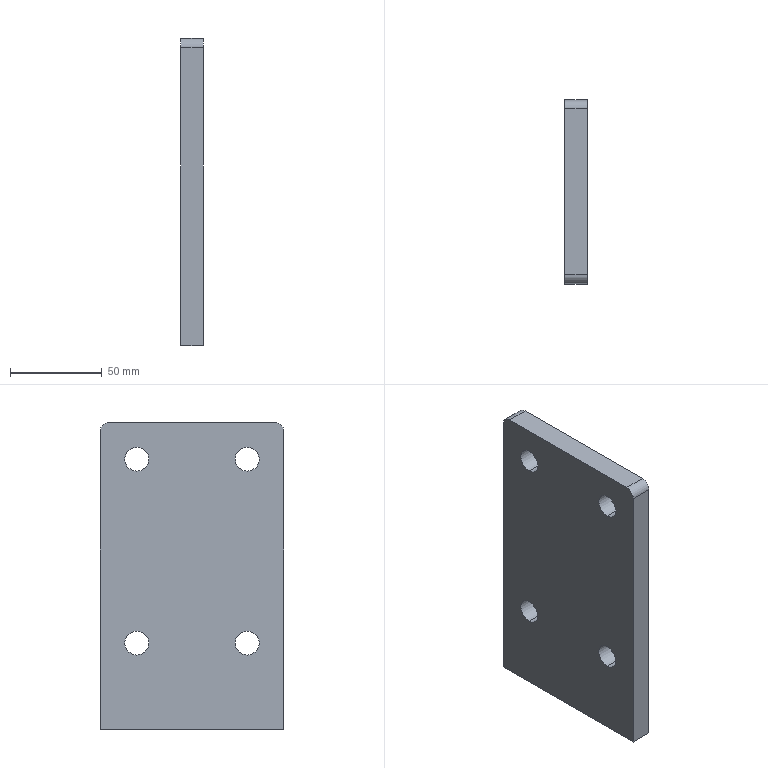Part | STEP file | 1 solid | 16 faces | box 12 x 100 x 167 mm | volume 193900 mm3 | cylinder 10 | plane 6 | commonest cylinder face diameters 13 x8 10 x2
STEP:
#1=CARTESIAN_POINT('',(0.,0.,0.));
#2=DIRECTION('',(0.,0.,1.));
#3=DIRECTION('',(1.,0.,0.));
#4=AXIS2_PLACEMENT_3D('',#1,#2,#3);
#5=CARTESIAN_POINT('',(-227.,-1110.,53.5));
#6=VERTEX_POINT('',#5);
#7=CARTESIAN_POINT('',(-227.,-1110.,40.5));
#8=VERTEX_POINT('',#7);
#9=CARTESIAN_POINT('',(-227.,-1110.,47.));
#10=DIRECTION('',(1.,0.,0.));
#11=DIRECTION('',(0.,0.,1.));
#12=AXIS2_PLACEMENT_3D('',#9,#10,#11);
#13=CIRCLE('',#12,6.5);
#14=CARTESIAN_POINT('',(-227.,-1030.,167.));
#15=DIRECTION('',(1.,0.,0.));
#16=DIRECTION('',(0.,1.,0.));
#17=AXIS2_PLACEMENT_3D('',#14,#15,#16);
#18=PLANE('',#17);
#19=CARTESIAN_POINT('',(-80.,-120.));
#20=DIRECTION('',(0.,1.));
#21=AXIS2_PLACEMENT_2D('',#19,#20);
#22=CIRCLE('',#21,6.5);
#23=(GEOMETRIC_REPRESENTATION_CONTEXT(2)PARAMETRIC_REPRESENTATION_CONTEXT()REPRESENTATION_CONTEXT('',''));
#24=DEFINITIONAL_REPRESENTATION('',(#22),#23);
#25=PCURVE('',#18,#24);
#26=CARTESIAN_POINT('',(-214.999,-1110.,47.));
#27=DIRECTION('',(-1.,0.,0.));
#28=DIRECTION('',(0.,0.,1.));
#29=AXIS2_PLACEMENT_3D('',#26,#27,#28);
#30=CYLINDRICAL_SURFACE('',#29,6.5);
#31=CARTESIAN_POINT('',(6.283,12.001));
#32=DIRECTION('',(-1.,0.));
#33=VECTOR('',#32,1.);
#34=LINE('',#31,#33);
#35=(GEOMETRIC_REPRESENTATION_CONTEXT(2)PARAMETRIC_REPRESENTATION_CONTEXT()REPRESENTATION_CONTEXT('',''));
#36=DEFINITIONAL_REPRESENTATION('',(#34),#35);
#37=PCURVE('',#30,#36);
#38=SURFACE_CURVE('',#13,(#25,#37),.PCURVE_S1.);
#39=EDGE_CURVE('',#6,#8,#38,.T.);
#40=ORIENTED_EDGE('',*,*,#39,.T.);
#41=CARTESIAN_POINT('',(-227.,-1110.,47.));
#42=DIRECTION('',(1.,0.,0.));
#43=DIRECTION('',(0.,0.,1.));
#44=AXIS2_PLACEMENT_3D('',#41,#42,#43);
#45=CIRCLE('',#44,6.5);
#46=CARTESIAN_POINT('',(-80.,-120.));
#47=DIRECTION('',(0.,1.));
#48=AXIS2_PLACEMENT_2D('',#46,#47);
#49=CIRCLE('',#48,6.5);
#50=(GEOMETRIC_REPRESENTATION_CONTEXT(2)PARAMETRIC_REPRESENTATION_CONTEXT()REPRESENTATION_CONTEXT('',''));
#51=DEFINITIONAL_REPRESENTATION('',(#49),#50);
#52=PCURVE('',#18,#51);
#53=CARTESIAN_POINT('',(-214.999,-1110.,47.));
#54=DIRECTION('',(-1.,0.,0.));
#55=DIRECTION('',(0.,0.,1.));
#56=AXIS2_PLACEMENT_3D('',#53,#54,#55);
#57=CYLINDRICAL_SURFACE('',#56,6.5);
#58=CARTESIAN_POINT('',(6.283,12.001));
#59=DIRECTION('',(-1.,0.));
#60=VECTOR('',#59,1.);
#61=LINE('',#58,#60);
#62=(GEOMETRIC_REPRESENTATION_CONTEXT(2)PARAMETRIC_REPRESENTATION_CONTEXT()REPRESENTATION_CONTEXT('',''));
#63=DEFINITIONAL_REPRESENTATION('',(#61),#62);
#64=PCURVE('',#57,#63);
#65=SURFACE_CURVE('',#45,(#52,#64),.PCURVE_S1.);
#66=EDGE_CURVE('',#8,#6,#65,.T.);
#67=ORIENTED_EDGE('',*,*,#66,.T.);
#68=EDGE_LOOP('',(#40,#67));
#69=FACE_BOUND('',#68,.T.);
#70=CARTESIAN_POINT('',(-227.,-1110.,153.5));
#71=VERTEX_POINT('',#70);
#72=CARTESIAN_POINT('',(-227.,-1110.,140.5));
#73=VERTEX_POINT('',#72);
#74=CARTESIAN_POINT('',(-227.,-1110.,147.));
#75=DIRECTION('',(1.,0.,0.));
#76=DIRECTION('',(0.,0.,1.));
#77=AXIS2_PLACEMENT_3D('',#74,#75,#76);
#78=CIRCLE('',#77,6.5);
#79=CARTESIAN_POINT('',(-80.,-20.));
#80=DIRECTION('',(0.,1.));
#81=AXIS2_PLACEMENT_2D('',#79,#80);
#82=CIRCLE('',#81,6.5);
#83=(GEOMETRIC_REPRESENTATION_CONTEXT(2)PARAMETRIC_REPRESENTATION_CONTEXT()REPRESENTATION_CONTEXT('',''));
#84=DEFINITIONAL_REPRESENTATION('',(#82),#83);
#85=PCURVE('',#18,#84);
#86=CARTESIAN_POINT('',(-214.999,-1110.,147.));
#87=DIRECTION('',(-1.,0.,0.));
#88=DIRECTION('',(0.,0.,1.));
#89=AXIS2_PLACEMENT_3D('',#86,#87,#88);
#90=CYLINDRICAL_SURFACE('',#89,6.5);
#91=CARTESIAN_POINT('',(6.283,12.001));
#92=DIRECTION('',(-1.,0.));
#93=VECTOR('',#92,1.);
#94=LINE('',#91,#93);
#95=(GEOMETRIC_REPRESENTATION_CONTEXT(2)PARAMETRIC_REPRESENTATION_CONTEXT()REPRESENTATION_CONTEXT('',''));
#96=DEFINITIONAL_REPRESENTATION('',(#94),#95);
#97=PCURVE('',#90,#96);
#98=SURFACE_CURVE('',#78,(#85,#97),.PCURVE_S1.);
#99=EDGE_CURVE('',#71,#73,#98,.T.);
#100=ORIENTED_EDGE('',*,*,#99,.T.);
#101=CARTESIAN_POINT('',(-227.,-1110.,147.));
#102=DIRECTION('',(1.,0.,0.));
#103=DIRECTION('',(0.,0.,1.));
#104=AXIS2_PLACEMENT_3D('',#101,#102,#103);
#105=CIRCLE('',#104,6.5);
#106=CARTESIAN_POINT('',(-80.,-20.));
#107=DIRECTION('',(0.,1.));
#108=AXIS2_PLACEMENT_2D('',#106,#107);
#109=CIRCLE('',#108,6.5);
#110=(GEOMETRIC_REPRESENTATION_CONTEXT(2)PARAMETRIC_REPRESENTATION_CONTEXT()REPRESENTATION_CONTEXT('',''));
#111=DEFINITIONAL_REPRESENTATION('',(#109),#110);
#112=PCURVE('',#18,#111);
#113=CARTESIAN_POINT('',(-214.999,-1110.,147.));
#114=DIRECTION('',(-1.,0.,0.));
#115=DIRECTION('',(0.,0.,1.));
#116=AXIS2_PLACEMENT_3D('',#113,#114,#115);
#117=CYLINDRICAL_SURFACE('',#116,6.5);
#118=CARTESIAN_POINT('',(6.283,12.001));
#119=DIRECTION('',(-1.,0.));
#120=VECTOR('',#119,1.);
#121=LINE('',#118,#120);
#122=(GEOMETRIC_REPRESENTATION_CONTEXT(2)PARAMETRIC_REPRESENTATION_CONTEXT()REPRESENTATION_CONTEXT('',''));
#123=DEFINITIONAL_REPRESENTATION('',(#121),#122);
#124=PCURVE('',#117,#123);
#125=SURFACE_CURVE('',#105,(#112,#124),.PCURVE_S1.);
#126=EDGE_CURVE('',#73,#71,#125,.T.);
#127=ORIENTED_EDGE('',*,*,#126,.T.);
#128=EDGE_LOOP('',(#100,#127));
#129=FACE_BOUND('',#128,.T.);
#130=CARTESIAN_POINT('',(-227.,-1050.,153.5));
#131=VERTEX_POINT('',#130);
#132=CARTESIAN_POINT('',(-227.,-1050.,140.5));
#133=VERTEX_POINT('',#132);
#134=CARTESIAN_POINT('',(-227.,-1050.,147.));
#135=DIRECTION('',(1.,0.,0.));
#136=DIRECTION('',(0.,0.,1.));
#137=AXIS2_PLACEMENT_3D('',#134,#135,#136);
#138=CIRCLE('',#137,6.5);
#139=CARTESIAN_POINT('',(-20.,-20.));
#140=DIRECTION('',(0.,1.));
#141=AXIS2_PLACEMENT_2D('',#139,#140);
#142=CIRCLE('',#141,6.5);
#143=(GEOMETRIC_REPRESENTATION_CONTEXT(2)PARAMETRIC_REPRESENTATION_CONTEXT()REPRESENTATION_CONTEXT('',''));
#144=DEFINITIONAL_REPRESENTATION('',(#142),#143);
#145=PCURVE('',#18,#144);
#146=CARTESIAN_POINT('',(-214.999,-1050.,147.));
#147=DIRECTION('',(-1.,0.,0.));
#148=DIRECTION('',(0.,0.,1.));
#149=AXIS2_PLACEMENT_3D('',#146,#147,#148);
#150=CYLINDRICAL_SURFACE('',#149,6.5);
#151=CARTESIAN_POINT('',(6.283,12.001));
#152=DIRECTION('',(-1.,0.));
#153=VECTOR('',#152,1.);
#154=LINE('',#151,#153);
#155=(GEOMETRIC_REPRESENTATION_CONTEXT(2)PARAMETRIC_REPRESENTATION_CONTEXT()REPRESENTATION_CONTEXT('',''));
#156=DEFINITIONAL_REPRESENTATION('',(#154),#155);
#157=PCURVE('',#150,#156);
#158=SURFACE_CURVE('',#138,(#145,#157),.PCURVE_S1.);
#159=EDGE_CURVE('',#131,#133,#158,.T.);
#160=ORIENTED_EDGE('',*,*,#159,.T.);
#161=CARTESIAN_POINT('',(-227.,-1050.,147.));
#162=DIRECTION('',(1.,0.,0.));
#163=DIRECTION('',(0.,0.,1.));
#164=AXIS2_PLACEMENT_3D('',#161,#162,#163);
#165=CIRCLE('',#164,6.5);
#166=CARTESIAN_POINT('',(-20.,-20.));
#167=DIRECTION('',(0.,1.));
#168=AXIS2_PLACEMENT_2D('',#166,#167);
#169=CIRCLE('',#168,6.5);
#170=(GEOMETRIC_REPRESENTATION_CONTEXT(2)PARAMETRIC_REPRESENTATION_CONTEXT()REPRESENTATION_CONTEXT('',''));
#171=DEFINITIONAL_REPRESENTATION('',(#169),#170);
#172=PCURVE('',#18,#171);
#173=CARTESIAN_POINT('',(-214.999,-1050.,147.));
#174=DIRECTION('',(-1.,0.,0.));
#175=DIRECTION('',(0.,0.,1.));
#176=AXIS2_PLACEMENT_3D('',#173,#174,#175);
#177=CYLINDRICAL_SURFACE('',#176,6.5);
#178=CARTESIAN_POINT('',(6.283,12.001));
#179=DIRECTION('',(-1.,0.));
#180=VECTOR('',#179,1.);
#181=LINE('',#178,#180);
#182=(GEOMETRIC_REPRESENTATION_CONTEXT(2)PARAMETRIC_REPRESENTATION_CONTEXT()REPRESENTATION_CONTEXT('',''));
#183=DEFINITIONAL_REPRESENTATION('',(#181),#182);
#184=PCURVE('',#177,#183);
#185=SURFACE_CURVE('',#165,(#172,#184),.PCURVE_S1.);
#186=EDGE_CURVE('',#133,#131,#185,.T.);
#187=ORIENTED_EDGE('',*,*,#186,.T.);
#188=EDGE_LOOP('',(#160,#187));
#189=FACE_BOUND('',#188,.T.);
#190=CARTESIAN_POINT('',(-227.,-1050.,53.5));
#191=VERTEX_POINT('',#190);
#192=CARTESIAN_POINT('',(-227.,-1050.,40.5));
#193=VERTEX_POINT('',#192);
#194=CARTESIAN_POINT('',(-227.,-1050.,47.));
#195=DIRECTION('',(1.,0.,0.));
#196=DIRECTION('',(0.,0.,1.));
#197=AXIS2_PLACEMENT_3D('',#194,#195,#196);
#198=CIRCLE('',#197,6.5);
#199=CARTESIAN_POINT('',(-20.,-120.));
#200=DIRECTION('',(0.,1.));
#201=AXIS2_PLACEMENT_2D('',#199,#200);
#202=CIRCLE('',#201,6.5);
#203=(GEOMETRIC_REPRESENTATION_CONTEXT(2)PARAMETRIC_REPRESENTATION_CONTEXT()REPRESENTATION_CONTEXT('',''));
#204=DEFINITIONAL_REPRESENTATION('',(#202),#203);
#205=PCURVE('',#18,#204);
#206=CARTESIAN_POINT('',(-214.999,-1050.,47.));
#207=DIRECTION('',(-1.,0.,0.));
#208=DIRECTION('',(0.,0.,1.));
#209=AXIS2_PLACEMENT_3D('',#206,#207,#208);
#210=CYLINDRICAL_SURFACE('',#209,6.5);
#211=CARTESIAN_POINT('',(6.283,12.001));
#212=DIRECTION('',(-1.,0.));
#213=VECTOR('',#212,1.);
#214=LINE('',#211,#213);
#215=(GEOMETRIC_REPRESENTATION_CONTEXT(2)PARAMETRIC_REPRESENTATION_CONTEXT()REPRESENTATION_CONTEXT('',''));
#216=DEFINITIONAL_REPRESENTATION('',(#214),#215);
#217=PCURVE('',#210,#216);
#218=SURFACE_CURVE('',#198,(#205,#217),.PCURVE_S1.);
#219=EDGE_CURVE('',#191,#193,#218,.T.);
#220=ORIENTED_EDGE('',*,*,#219,.T.);
#221=CARTESIAN_POINT('',(-227.,-1050.,47.));
#222=DIRECTION('',(1.,0.,0.));
#223=DIRECTION('',(0.,0.,1.));
#224=AXIS2_PLACEMENT_3D('',#221,#222,#223);
#225=CIRCLE('',#224,6.5);
#226=CARTESIAN_POINT('',(-20.,-120.));
#227=DIRECTION('',(0.,1.));
#228=AXIS2_PLACEMENT_2D('',#226,#227);
#229=CIRCLE('',#228,6.5);
#230=(GEOMETRIC_REPRESENTATION_CONTEXT(2)PARAMETRIC_REPRESENTATION_CONTEXT()REPRESENTATION_CONTEXT('',''));
#231=DEFINITIONAL_REPRESENTATION('',(#229),#230);
#232=PCURVE('',#18,#231);
#233=CARTESIAN_POINT('',(-214.999,-1050.,47.));
#234=DIRECTION('',(-1.,0.,0.));
#235=DIRECTION('',(0.,0.,1.));
#236=AXIS2_PLACEMENT_3D('',#233,#234,#235);
#237=CYLINDRICAL_SURFACE('',#236,6.5);
#238=CARTESIAN_POINT('',(6.283,12.001));
#239=DIRECTION('',(-1.,0.));
#240=VECTOR('',#239,1.);
#241=LINE('',#238,#240);
#242=(GEOMETRIC_REPRESENTATION_CONTEXT(2)PARAMETRIC_REPRESENTATION_CONTEXT()REPRESENTATION_CONTEXT('',''));
#243=DEFINITIONAL_REPRESENTATION('',(#241),#242);
#244=PCURVE('',#237,#243);
#245=SURFACE_CURVE('',#225,(#232,#244),.PCURVE_S1.);
#246=EDGE_CURVE('',#193,#191,#245,.T.);
#247=ORIENTED_EDGE('',*,*,#246,.T.);
#248=EDGE_LOOP('',(#220,#247));
#249=FACE_BOUND('',#248,.T.);
#250=CARTESIAN_POINT('',(-227.,-1125.,167.));
#251=VERTEX_POINT('',#250);
#252=CARTESIAN_POINT('',(-227.,-1130.,162.));
#253=VERTEX_POINT('',#252);
#254=CARTESIAN_POINT('',(-227.,-1125.,162.));
#255=DIRECTION('',(1.,0.,0.));
#256=DIRECTION('',(0.,0.,1.));
#257=AXIS2_PLACEMENT_3D('',#254,#255,#256);
#258=CIRCLE('',#257,5.);
#259=CARTESIAN_POINT('',(-95.,-5.));
#260=DIRECTION('',(0.,1.));
#261=AXIS2_PLACEMENT_2D('',#259,#260);
#262=CIRCLE('',#261,5.);
#263=(GEOMETRIC_REPRESENTATION_CONTEXT(2)PARAMETRIC_REPRESENTATION_CONTEXT()REPRESENTATION_CONTEXT('',''));
#264=DEFINITIONAL_REPRESENTATION('',(#262),#263);
#265=PCURVE('',#18,#264);
#266=CARTESIAN_POINT('',(0.,-1125.,162.));
#267=DIRECTION('',(-1.,0.,0.));
#268=DIRECTION('',(0.,0.,1.));
#269=AXIS2_PLACEMENT_3D('',#266,#267,#268);
#270=CYLINDRICAL_SURFACE('',#269,5.);
#271=CARTESIAN_POINT('',(6.283,227.));
#272=DIRECTION('',(-1.,0.));
#273=VECTOR('',#272,1.);
#274=LINE('',#271,#273);
#275=(GEOMETRIC_REPRESENTATION_CONTEXT(2)PARAMETRIC_REPRESENTATION_CONTEXT()REPRESENTATION_CONTEXT('',''));
#276=DEFINITIONAL_REPRESENTATION('',(#274),#275);
#277=PCURVE('',#270,#276);
#278=SURFACE_CURVE('',#258,(#265,#277),.PCURVE_S1.);
#279=EDGE_CURVE('',#251,#253,#278,.T.);
#280=ORIENTED_EDGE('',*,*,#279,.F.);
#281=CARTESIAN_POINT('',(-227.,-1035.,167.));
#282=VERTEX_POINT('',#281);
#283=CARTESIAN_POINT('',(-227.,0.,167.));
#284=DIRECTION('',(0.,-1.,0.));
#285=VECTOR('',#284,1.);
#286=LINE('',#283,#285);
#287=CARTESIAN_POINT('',(1030.,0.));
#288=DIRECTION('',(-1.,0.));
#289=VECTOR('',#288,1.);
#290=LINE('',#287,#289);
#291=(GEOMETRIC_REPRESENTATION_CONTEXT(2)PARAMETRIC_REPRESENTATION_CONTEXT()REPRESENTATION_CONTEXT('',''));
#292=DEFINITIONAL_REPRESENTATION('',(#290),#291);
#293=PCURVE('',#18,#292);
#294=CARTESIAN_POINT('',(0.,0.,167.));
#295=DIRECTION('',(0.,0.,1.));
#296=DIRECTION('',(1.,0.,0.));
#297=AXIS2_PLACEMENT_3D('',#294,#295,#296);
#298=PLANE('',#297);
#299=CARTESIAN_POINT('',(-227.,0.));
#300=DIRECTION('',(0.,-1.));
#301=VECTOR('',#300,1.);
#302=LINE('',#299,#301);
#303=(GEOMETRIC_REPRESENTATION_CONTEXT(2)PARAMETRIC_REPRESENTATION_CONTEXT()REPRESENTATION_CONTEXT('',''));
#304=DEFINITIONAL_REPRESENTATION('',(#302),#303);
#305=PCURVE('',#298,#304);
#306=SURFACE_CURVE('',#286,(#293,#305),.PCURVE_S1.);
#307=EDGE_CURVE('',#282,#251,#306,.T.);
#308=ORIENTED_EDGE('',*,*,#307,.F.);
#309=CARTESIAN_POINT('',(-227.,-1030.,162.));
#310=VERTEX_POINT('',#309);
#311=CARTESIAN_POINT('',(-227.,-1035.,162.));
#312=DIRECTION('',(1.,0.,0.));
#313=DIRECTION('',(0.,0.,-1.));
#314=AXIS2_PLACEMENT_3D('',#311,#312,#313);
#315=CIRCLE('',#314,5.);
#316=CARTESIAN_POINT('',(-5.,-5.));
#317=DIRECTION('',(0.,-1.));
#318=AXIS2_PLACEMENT_2D('',#316,#317);
#319=CIRCLE('',#318,5.);
#320=(GEOMETRIC_REPRESENTATION_CONTEXT(2)PARAMETRIC_REPRESENTATION_CONTEXT()REPRESENTATION_CONTEXT('',''));
#321=DEFINITIONAL_REPRESENTATION('',(#319),#320);
#322=PCURVE('',#18,#321);
#323=CARTESIAN_POINT('',(0.,-1035.,162.));
#324=DIRECTION('',(1.,0.,0.));
#325=DIRECTION('',(0.,0.,-1.));
#326=AXIS2_PLACEMENT_3D('',#323,#324,#325);
#327=CYLINDRICAL_SURFACE('',#326,5.);
#328=CARTESIAN_POINT('',(0.,-227.));
#329=DIRECTION('',(1.,0.));
#330=VECTOR('',#329,1.);
#331=LINE('',#328,#330);
#332=(GEOMETRIC_REPRESENTATION_CONTEXT(2)PARAMETRIC_REPRESENTATION_CONTEXT()REPRESENTATION_CONTEXT('',''));
#333=DEFINITIONAL_REPRESENTATION('',(#331),#332);
#334=PCURVE('',#327,#333);
#335=SURFACE_CURVE('',#315,(#322,#334),.PCURVE_S1.);
#336=EDGE_CURVE('',#310,#282,#335,.T.);
#337=ORIENTED_EDGE('',*,*,#336,.F.);
#338=CARTESIAN_POINT('',(-227.,-1030.,0.));
#339=VERTEX_POINT('',#338);
#340=CARTESIAN_POINT('',(-227.,-1030.,167.));
#341=DIRECTION('',(0.,0.,-1.));
#342=VECTOR('',#341,1.);
#343=LINE('',#340,#342);
#344=CARTESIAN_POINT('',(0.,0.));
#345=DIRECTION('',(0.,-1.));
#346=VECTOR('',#345,1.);
#347=LINE('',#344,#346);
#348=(GEOMETRIC_REPRESENTATION_CONTEXT(2)PARAMETRIC_REPRESENTATION_CONTEXT()REPRESENTATION_CONTEXT('',''));
#349=DEFINITIONAL_REPRESENTATION('',(#347),#348);
#350=PCURVE('',#18,#349);
#351=CARTESIAN_POINT('',(-227.,-1030.,167.));
#352=DIRECTION('',(0.,-1.,0.));
#353=DIRECTION('',(0.,0.,-1.));
#354=AXIS2_PLACEMENT_3D('',#351,#352,#353);
#355=PLANE('',#354);
#356=CARTESIAN_POINT('',(0.,0.));
#357=DIRECTION('',(1.,0.));
#358=VECTOR('',#357,1.);
#359=LINE('',#356,#358);
#360=(GEOMETRIC_REPRESENTATION_CONTEXT(2)PARAMETRIC_REPRESENTATION_CONTEXT()REPRESENTATION_CONTEXT('',''));
#361=DEFINITIONAL_REPRESENTATION('',(#359),#360);
#362=PCURVE('',#355,#361);
#363=SURFACE_CURVE('',#343,(#350,#362),.PCURVE_S1.);
#364=EDGE_CURVE('',#310,#339,#363,.T.);
#365=ORIENTED_EDGE('',*,*,#364,.T.);
#366=CARTESIAN_POINT('',(-227.,-1130.,0.));
#367=VERTEX_POINT('',#366);
#368=CARTESIAN_POINT('',(-227.,0.,0.));
#369=DIRECTION('',(0.,-1.,0.));
#370=VECTOR('',#369,1.);
#371=LINE('',#368,#370);
#372=CARTESIAN_POINT('',(1030.,-167.));
#373=DIRECTION('',(-1.,0.));
#374=VECTOR('',#373,1.);
#375=LINE('',#372,#374);
#376=(GEOMETRIC_REPRESENTATION_CONTEXT(2)PARAMETRIC_REPRESENTATION_CONTEXT()REPRESENTATION_CONTEXT('',''));
#377=DEFINITIONAL_REPRESENTATION('',(#375),#376);
#378=PCURVE('',#18,#377);
#379=CARTESIAN_POINT('',(0.,0.,0.));
#380=DIRECTION('',(0.,0.,1.));
#381=DIRECTION('',(1.,0.,0.));
#382=AXIS2_PLACEMENT_3D('',#379,#380,#381);
#383=PLANE('',#382);
#384=CARTESIAN_POINT('',(-227.,0.));
#385=DIRECTION('',(0.,-1.));
#386=VECTOR('',#385,1.);
#387=LINE('',#384,#386);
#388=(GEOMETRIC_REPRESENTATION_CONTEXT(2)PARAMETRIC_REPRESENTATION_CONTEXT()REPRESENTATION_CONTEXT('',''));
#389=DEFINITIONAL_REPRESENTATION('',(#387),#388);
#390=PCURVE('',#383,#389);
#391=SURFACE_CURVE('',#371,(#378,#390),.PCURVE_S1.);
#392=EDGE_CURVE('',#339,#367,#391,.T.);
#393=ORIENTED_EDGE('',*,*,#392,.T.);
#394=CARTESIAN_POINT('',(-227.,-1130.,167.));
#395=DIRECTION('',(0.,0.,1.));
#396=VECTOR('',#395,1.);
#397=LINE('',#394,#396);
#398=CARTESIAN_POINT('',(-100.,0.));
#399=DIRECTION('',(0.,1.));
#400=VECTOR('',#399,1.);
#401=LINE('',#398,#400);
#402=(GEOMETRIC_REPRESENTATION_CONTEXT(2)PARAMETRIC_REPRESENTATION_CONTEXT()REPRESENTATION_CONTEXT('',''));
#403=DEFINITIONAL_REPRESENTATION('',(#401),#402);
#404=PCURVE('',#18,#403);
#405=CARTESIAN_POINT('',(-227.,-1130.,167.));
#406=DIRECTION('',(0.,1.,0.));
#407=DIRECTION('',(1.,0.,0.));
#408=AXIS2_PLACEMENT_3D('',#405,#406,#407);
#409=PLANE('',#408);
#410=CARTESIAN_POINT('',(0.,0.));
#411=DIRECTION('',(0.,-1.));
#412=VECTOR('',#411,1.);
#413=LINE('',#410,#412);
#414=(GEOMETRIC_REPRESENTATION_CONTEXT(2)PARAMETRIC_REPRESENTATION_CONTEXT()REPRESENTATION_CONTEXT('',''));
#415=DEFINITIONAL_REPRESENTATION('',(#413),#414);
#416=PCURVE('',#409,#415);
#417=SURFACE_CURVE('',#397,(#404,#416),.PCURVE_S1.);
#418=EDGE_CURVE('',#367,#253,#417,.T.);
#419=ORIENTED_EDGE('',*,*,#418,.T.);
#420=EDGE_LOOP('',(#280,#308,#337,#365,#393,#419));
#421=FACE_BOUND('',#420,.T.);
#422=ADVANCED_FACE('',(#69,#129,#189,#249,#421),#18,.F.);
#423=ORIENTED_EDGE('',*,*,#66,.T.);
#424=CARTESIAN_POINT('',(-215.,-1110.,53.5));
#425=VERTEX_POINT('',#424);
#426=CARTESIAN_POINT('',(-214.999,-1110.,53.5));
#427=DIRECTION('',(-1.,0.,0.));
#428=VECTOR('',#427,1.);
#429=LINE('',#426,#428);
#430=CARTESIAN_POINT('',(0.,0.));
#431=DIRECTION('',(0.,1.));
#432=VECTOR('',#431,1.);
#433=LINE('',#430,#432);
#434=(GEOMETRIC_REPRESENTATION_CONTEXT(2)PARAMETRIC_REPRESENTATION_CONTEXT()REPRESENTATION_CONTEXT('',''));
#435=DEFINITIONAL_REPRESENTATION('',(#433),#434);
#436=PCURVE('',#57,#435);
#437=CARTESIAN_POINT('',(6.283,0.));
#438=DIRECTION('',(0.,1.));
#439=VECTOR('',#438,1.);
#440=LINE('',#437,#439);
#441=(GEOMETRIC_REPRESENTATION_CONTEXT(2)PARAMETRIC_REPRESENTATION_CONTEXT()REPRESENTATION_CONTEXT('',''));
#442=DEFINITIONAL_REPRESENTATION('',(#440),#441);
#443=PCURVE('',#30,#442);
#444=SURFACE_CURVE('',#429,(#436,#443),.PCURVE_S1.);
#445=EDGE_CURVE('',#425,#6,#444,.T.);
#446=ORIENTED_EDGE('',*,*,#445,.F.);
#447=CARTESIAN_POINT('',(-215.,-1110.,40.5));
#448=VERTEX_POINT('',#447);
#449=CARTESIAN_POINT('',(-215.,-1110.,47.));
#450=DIRECTION('',(1.,0.,0.));
#451=DIRECTION('',(0.,0.,1.));
#452=AXIS2_PLACEMENT_3D('',#449,#450,#451);
#453=CIRCLE('',#452,6.5);
#454=CARTESIAN_POINT('',(6.283,0.001));
#455=DIRECTION('',(-1.,0.));
#456=VECTOR('',#455,1.);
#457=LINE('',#454,#456);
#458=(GEOMETRIC_REPRESENTATION_CONTEXT(2)PARAMETRIC_REPRESENTATION_CONTEXT()REPRESENTATION_CONTEXT('',''));
#459=DEFINITIONAL_REPRESENTATION('',(#457),#458);
#460=PCURVE('',#57,#459);
#461=CARTESIAN_POINT('',(-215.,-1030.,167.));
#462=DIRECTION('',(-1.,0.,0.));
#463=DIRECTION('',(0.,0.,1.));
#464=AXIS2_PLACEMENT_3D('',#461,#462,#463);
#465=PLANE('',#464);
#466=CARTESIAN_POINT('',(-113.5,-80.));
#467=CARTESIAN_POINT('',(-113.5,-91.258));
#468=CARTESIAN_POINT('',(-123.25,-85.629));
#469=CARTESIAN_POINT('',(-133.,-80.));
#470=CARTESIAN_POINT('',(-123.25,-74.371));
#471=CARTESIAN_POINT('',(-113.5,-68.742));
#472=CARTESIAN_POINT('',(-113.5,-80.));
#473=(BOUNDED_CURVE()B_SPLINE_CURVE(2,(#466,#467,#468,#469,#470,#471,#472),.UNSPECIFIED.,.T.,.F.)B_SPLINE_CURVE_WITH_KNOTS((1,2,2,2,2,1),(-2.094,0.,2.094,4.189,6.283,8.378),.UNSPECIFIED.)CURVE()GEOMETRIC_REPRESENTATION_ITEM()RATIONAL_B_SPLINE_CURVE((1.,0.5,1.,0.5,1.,0.5,1.))REPRESENTATION_ITEM(''));
#474=(GEOMETRIC_REPRESENTATION_CONTEXT(2)PARAMETRIC_REPRESENTATION_CONTEXT()REPRESENTATION_CONTEXT('',''));
#475=DEFINITIONAL_REPRESENTATION('',(#473),#474);
#476=PCURVE('',#465,#475);
#477=SURFACE_CURVE('',#453,(#460,#476),.PCURVE_S1.);
#478=EDGE_CURVE('',#448,#425,#477,.T.);
#479=ORIENTED_EDGE('',*,*,#478,.F.);
#480=CARTESIAN_POINT('',(-214.999,-1110.,40.5));
#481=DIRECTION('',(-1.,0.,0.));
#482=VECTOR('',#481,1.);
#483=LINE('',#480,#482);
#484=CARTESIAN_POINT('',(3.142,0.));
#485=DIRECTION('',(0.,1.));
#486=VECTOR('',#485,1.);
#487=LINE('',#484,#486);
#488=(GEOMETRIC_REPRESENTATION_CONTEXT(2)PARAMETRIC_REPRESENTATION_CONTEXT()REPRESENTATION_CONTEXT('',''));
#489=DEFINITIONAL_REPRESENTATION('',(#487),#488);
#490=PCURVE('',#57,#489);
#491=CARTESIAN_POINT('',(3.142,0.));
#492=DIRECTION('',(0.,1.));
#493=VECTOR('',#492,1.);
#494=LINE('',#491,#493);
#495=(GEOMETRIC_REPRESENTATION_CONTEXT(2)PARAMETRIC_REPRESENTATION_CONTEXT()REPRESENTATION_CONTEXT('',''));
#496=DEFINITIONAL_REPRESENTATION('',(#494),#495);
#497=PCURVE('',#30,#496);
#498=SURFACE_CURVE('',#483,(#490,#497),.PCURVE_S1.);
#499=EDGE_CURVE('',#448,#8,#498,.T.);
#500=ORIENTED_EDGE('',*,*,#499,.T.);
#501=EDGE_LOOP('',(#423,#446,#479,#500));
#502=FACE_BOUND('',#501,.F.);
#503=ADVANCED_FACE('',(#502),#57,.F.);
#504=ORIENTED_EDGE('',*,*,#126,.T.);
#505=CARTESIAN_POINT('',(-215.,-1110.,153.5));
#506=VERTEX_POINT('',#505);
#507=CARTESIAN_POINT('',(-214.999,-1110.,153.5));
#508=DIRECTION('',(-1.,0.,0.));
#509=VECTOR('',#508,1.);
#510=LINE('',#507,#509);
#511=CARTESIAN_POINT('',(0.,0.));
#512=DIRECTION('',(0.,1.));
#513=VECTOR('',#512,1.);
#514=LINE('',#511,#513);
#515=(GEOMETRIC_REPRESENTATION_CONTEXT(2)PARAMETRIC_REPRESENTATION_CONTEXT()REPRESENTATION_CONTEXT('',''));
#516=DEFINITIONAL_REPRESENTATION('',(#514),#515);
#517=PCURVE('',#117,#516);
#518=CARTESIAN_POINT('',(6.283,0.));
#519=DIRECTION('',(0.,1.));
#520=VECTOR('',#519,1.);
#521=LINE('',#518,#520);
#522=(GEOMETRIC_REPRESENTATION_CONTEXT(2)PARAMETRIC_REPRESENTATION_CONTEXT()REPRESENTATION_CONTEXT('',''));
#523=DEFINITIONAL_REPRESENTATION('',(#521),#522);
#524=PCURVE('',#90,#523);
#525=SURFACE_CURVE('',#510,(#517,#524),.PCURVE_S1.);
#526=EDGE_CURVE('',#506,#71,#525,.T.);
#527=ORIENTED_EDGE('',*,*,#526,.F.);
#528=CARTESIAN_POINT('',(-215.,-1110.,140.5));
#529=VERTEX_POINT('',#528);
#530=CARTESIAN_POINT('',(-215.,-1110.,147.));
#531=DIRECTION('',(1.,0.,0.));
#532=DIRECTION('',(0.,0.,1.));
#533=AXIS2_PLACEMENT_3D('',#530,#531,#532);
#534=CIRCLE('',#533,6.5);
#535=CARTESIAN_POINT('',(6.283,0.001));
#536=DIRECTION('',(-1.,0.));
#537=VECTOR('',#536,1.);
#538=LINE('',#535,#537);
#539=(GEOMETRIC_REPRESENTATION_CONTEXT(2)PARAMETRIC_REPRESENTATION_CONTEXT()REPRESENTATION_CONTEXT('',''));
#540=DEFINITIONAL_REPRESENTATION('',(#538),#539);
#541=PCURVE('',#117,#540);
#542=CARTESIAN_POINT('',(-13.5,-80.));
#543=CARTESIAN_POINT('',(-13.5,-91.258));
#544=CARTESIAN_POINT('',(-23.25,-85.629));
#545=CARTESIAN_POINT('',(-33.,-80.));
#546=CARTESIAN_POINT('',(-23.25,-74.371));
#547=CARTESIAN_POINT('',(-13.5,-68.742));
#548=CARTESIAN_POINT('',(-13.5,-80.));
#549=(BOUNDED_CURVE()B_SPLINE_CURVE(2,(#542,#543,#544,#545,#546,#547,#548),.UNSPECIFIED.,.T.,.F.)B_SPLINE_CURVE_WITH_KNOTS((1,2,2,2,2,1),(-2.094,0.,2.094,4.189,6.283,8.378),.UNSPECIFIED.)CURVE()GEOMETRIC_REPRESENTATION_ITEM()RATIONAL_B_SPLINE_CURVE((1.,0.5,1.,0.5,1.,0.5,1.))REPRESENTATION_ITEM(''));
#550=(GEOMETRIC_REPRESENTATION_CONTEXT(2)PARAMETRIC_REPRESENTATION_CONTEXT()REPRESENTATION_CONTEXT('',''));
#551=DEFINITIONAL_REPRESENTATION('',(#549),#550);
#552=PCURVE('',#465,#551);
#553=SURFACE_CURVE('',#534,(#541,#552),.PCURVE_S1.);
#554=EDGE_CURVE('',#529,#506,#553,.T.);
#555=ORIENTED_EDGE('',*,*,#554,.F.);
#556=CARTESIAN_POINT('',(-214.999,-1110.,140.5));
#557=DIRECTION('',(-1.,0.,0.));
#558=VECTOR('',#557,1.);
#559=LINE('',#556,#558);
#560=CARTESIAN_POINT('',(3.142,0.));
#561=DIRECTION('',(0.,1.));
#562=VECTOR('',#561,1.);
#563=LINE('',#560,#562);
#564=(GEOMETRIC_REPRESENTATION_CONTEXT(2)PARAMETRIC_REPRESENTATION_CONTEXT()REPRESENTATION_CONTEXT('',''));
#565=DEFINITIONAL_REPRESENTATION('',(#563),#564);
#566=PCURVE('',#117,#565);
#567=CARTESIAN_POINT('',(3.142,0.));
#568=DIRECTION('',(0.,1.));
#569=VECTOR('',#568,1.);
#570=LINE('',#567,#569);
#571=(GEOMETRIC_REPRESENTATION_CONTEXT(2)PARAMETRIC_REPRESENTATION_CONTEXT()REPRESENTATION_CONTEXT('',''));
#572=DEFINITIONAL_REPRESENTATION('',(#570),#571);
#573=PCURVE('',#90,#572);
#574=SURFACE_CURVE('',#559,(#566,#573),.PCURVE_S1.);
#575=EDGE_CURVE('',#529,#73,#574,.T.);
#576=ORIENTED_EDGE('',*,*,#575,.T.);
#577=EDGE_LOOP('',(#504,#527,#555,#576));
#578=FACE_BOUND('',#577,.F.);
#579=ADVANCED_FACE('',(#578),#117,.F.);
#580=ORIENTED_EDGE('',*,*,#186,.T.);
#581=CARTESIAN_POINT('',(-215.,-1050.,153.5));
#582=VERTEX_POINT('',#581);
#583=CARTESIAN_POINT('',(-214.999,-1050.,153.5));
#584=DIRECTION('',(-1.,0.,0.));
#585=VECTOR('',#584,1.);
#586=LINE('',#583,#585);
#587=CARTESIAN_POINT('',(0.,0.));
#588=DIRECTION('',(0.,1.));
#589=VECTOR('',#588,1.);
#590=LINE('',#587,#589);
#591=(GEOMETRIC_REPRESENTATION_CONTEXT(2)PARAMETRIC_REPRESENTATION_CONTEXT()REPRESENTATION_CONTEXT('',''));
#592=DEFINITIONAL_REPRESENTATION('',(#590),#591);
#593=PCURVE('',#177,#592);
#594=CARTESIAN_POINT('',(6.283,0.));
#595=DIRECTION('',(0.,1.));
#596=VECTOR('',#595,1.);
#597=LINE('',#594,#596);
#598=(GEOMETRIC_REPRESENTATION_CONTEXT(2)PARAMETRIC_REPRESENTATION_CONTEXT()REPRESENTATION_CONTEXT('',''));
#599=DEFINITIONAL_REPRESENTATION('',(#597),#598);
#600=PCURVE('',#150,#599);
#601=SURFACE_CURVE('',#586,(#593,#600),.PCURVE_S1.);
#602=EDGE_CURVE('',#582,#131,#601,.T.);
#603=ORIENTED_EDGE('',*,*,#602,.F.);
#604=CARTESIAN_POINT('',(-215.,-1050.,140.5));
#605=VERTEX_POINT('',#604);
#606=CARTESIAN_POINT('',(-215.,-1050.,147.));
#607=DIRECTION('',(1.,0.,0.));
#608=DIRECTION('',(0.,0.,1.));
#609=AXIS2_PLACEMENT_3D('',#606,#607,#608);
#610=CIRCLE('',#609,6.5);
#611=CARTESIAN_POINT('',(6.283,0.001));
#612=DIRECTION('',(-1.,0.));
#613=VECTOR('',#612,1.);
#614=LINE('',#611,#613);
#615=(GEOMETRIC_REPRESENTATION_CONTEXT(2)PARAMETRIC_REPRESENTATION_CONTEXT()REPRESENTATION_CONTEXT('',''));
#616=DEFINITIONAL_REPRESENTATION('',(#614),#615);
#617=PCURVE('',#177,#616);
#618=CARTESIAN_POINT('',(-13.5,-20.));
#619=CARTESIAN_POINT('',(-13.5,-31.258));
#620=CARTESIAN_POINT('',(-23.25,-25.629));
#621=CARTESIAN_POINT('',(-33.,-20.));
#622=CARTESIAN_POINT('',(-23.25,-14.371));
#623=CARTESIAN_POINT('',(-13.5,-8.742));
#624=CARTESIAN_POINT('',(-13.5,-20.));
#625=(BOUNDED_CURVE()B_SPLINE_CURVE(2,(#618,#619,#620,#621,#622,#623,#624),.UNSPECIFIED.,.T.,.F.)B_SPLINE_CURVE_WITH_KNOTS((1,2,2,2,2,1),(-2.094,0.,2.094,4.189,6.283,8.378),.UNSPECIFIED.)CURVE()GEOMETRIC_REPRESENTATION_ITEM()RATIONAL_B_SPLINE_CURVE((1.,0.5,1.,0.5,1.,0.5,1.))REPRESENTATION_ITEM(''));
#626=(GEOMETRIC_REPRESENTATION_CONTEXT(2)PARAMETRIC_REPRESENTATION_CONTEXT()REPRESENTATION_CONTEXT('',''));
#627=DEFINITIONAL_REPRESENTATION('',(#625),#626);
#628=PCURVE('',#465,#627);
#629=SURFACE_CURVE('',#610,(#617,#628),.PCURVE_S1.);
#630=EDGE_CURVE('',#605,#582,#629,.T.);
#631=ORIENTED_EDGE('',*,*,#630,.F.);
#632=CARTESIAN_POINT('',(-214.999,-1050.,140.5));
#633=DIRECTION('',(-1.,0.,0.));
#634=VECTOR('',#633,1.);
#635=LINE('',#632,#634);
#636=CARTESIAN_POINT('',(3.142,0.));
#637=DIRECTION('',(0.,1.));
#638=VECTOR('',#637,1.);
#639=LINE('',#636,#638);
#640=(GEOMETRIC_REPRESENTATION_CONTEXT(2)PARAMETRIC_REPRESENTATION_CONTEXT()REPRESENTATION_CONTEXT('',''));
#641=DEFINITIONAL_REPRESENTATION('',(#639),#640);
#642=PCURVE('',#177,#641);
#643=CARTESIAN_POINT('',(3.142,0.));
#644=DIRECTION('',(0.,1.));
#645=VECTOR('',#644,1.);
#646=LINE('',#643,#645);
#647=(GEOMETRIC_REPRESENTATION_CONTEXT(2)PARAMETRIC_REPRESENTATION_CONTEXT()REPRESENTATION_CONTEXT('',''));
#648=DEFINITIONAL_REPRESENTATION('',(#646),#647);
#649=PCURVE('',#150,#648);
#650=SURFACE_CURVE('',#635,(#642,#649),.PCURVE_S1.);
#651=EDGE_CURVE('',#605,#133,#650,.T.);
#652=ORIENTED_EDGE('',*,*,#651,.T.);
#653=EDGE_LOOP('',(#580,#603,#631,#652));
#654=FACE_BOUND('',#653,.F.);
#655=ADVANCED_FACE('',(#654),#177,.F.);
#656=ORIENTED_EDGE('',*,*,#246,.T.);
#657=CARTESIAN_POINT('',(-215.,-1050.,53.5));
#658=VERTEX_POINT('',#657);
#659=CARTESIAN_POINT('',(-214.999,-1050.,53.5));
#660=DIRECTION('',(-1.,0.,0.));
#661=VECTOR('',#660,1.);
#662=LINE('',#659,#661);
#663=CARTESIAN_POINT('',(0.,0.));
#664=DIRECTION('',(0.,1.));
#665=VECTOR('',#664,1.);
#666=LINE('',#663,#665);
#667=(GEOMETRIC_REPRESENTATION_CONTEXT(2)PARAMETRIC_REPRESENTATION_CONTEXT()REPRESENTATION_CONTEXT('',''));
#668=DEFINITIONAL_REPRESENTATION('',(#666),#667);
#669=PCURVE('',#237,#668);
#670=CARTESIAN_POINT('',(6.283,0.));
#671=DIRECTION('',(0.,1.));
#672=VECTOR('',#671,1.);
#673=LINE('',#670,#672);
#674=(GEOMETRIC_REPRESENTATION_CONTEXT(2)PARAMETRIC_REPRESENTATION_CONTEXT()REPRESENTATION_CONTEXT('',''));
#675=DEFINITIONAL_REPRESENTATION('',(#673),#674);
#676=PCURVE('',#210,#675);
#677=SURFACE_CURVE('',#662,(#669,#676),.PCURVE_S1.);
#678=EDGE_CURVE('',#658,#191,#677,.T.);
#679=ORIENTED_EDGE('',*,*,#678,.F.);
#680=CARTESIAN_POINT('',(-215.,-1050.,40.5));
#681=VERTEX_POINT('',#680);
#682=CARTESIAN_POINT('',(-215.,-1050.,47.));
#683=DIRECTION('',(1.,0.,0.));
#684=DIRECTION('',(0.,0.,1.));
#685=AXIS2_PLACEMENT_3D('',#682,#683,#684);
#686=CIRCLE('',#685,6.5);
#687=CARTESIAN_POINT('',(6.283,0.001));
#688=DIRECTION('',(-1.,0.));
#689=VECTOR('',#688,1.);
#690=LINE('',#687,#689);
#691=(GEOMETRIC_REPRESENTATION_CONTEXT(2)PARAMETRIC_REPRESENTATION_CONTEXT()REPRESENTATION_CONTEXT('',''));
#692=DEFINITIONAL_REPRESENTATION('',(#690),#691);
#693=PCURVE('',#237,#692);
#694=CARTESIAN_POINT('',(-113.5,-20.));
#695=CARTESIAN_POINT('',(-113.5,-31.258));
#696=CARTESIAN_POINT('',(-123.25,-25.629));
#697=CARTESIAN_POINT('',(-133.,-20.));
#698=CARTESIAN_POINT('',(-123.25,-14.371));
#699=CARTESIAN_POINT('',(-113.5,-8.742));
#700=CARTESIAN_POINT('',(-113.5,-20.));
#701=(BOUNDED_CURVE()B_SPLINE_CURVE(2,(#694,#695,#696,#697,#698,#699,#700),.UNSPECIFIED.,.T.,.F.)B_SPLINE_CURVE_WITH_KNOTS((1,2,2,2,2,1),(-2.094,0.,2.094,4.189,6.283,8.378),.UNSPECIFIED.)CURVE()GEOMETRIC_REPRESENTATION_ITEM()RATIONAL_B_SPLINE_CURVE((1.,0.5,1.,0.5,1.,0.5,1.))REPRESENTATION_ITEM(''));
#702=(GEOMETRIC_REPRESENTATION_CONTEXT(2)PARAMETRIC_REPRESENTATION_CONTEXT()REPRESENTATION_CONTEXT('',''));
#703=DEFINITIONAL_REPRESENTATION('',(#701),#702);
#704=PCURVE('',#465,#703);
#705=SURFACE_CURVE('',#686,(#693,#704),.PCURVE_S1.);
#706=EDGE_CURVE('',#681,#658,#705,.T.);
#707=ORIENTED_EDGE('',*,*,#706,.F.);
#708=CARTESIAN_POINT('',(-214.999,-1050.,40.5));
#709=DIRECTION('',(-1.,0.,0.));
#710=VECTOR('',#709,1.);
#711=LINE('',#708,#710);
#712=CARTESIAN_POINT('',(3.142,0.));
#713=DIRECTION('',(0.,1.));
#714=VECTOR('',#713,1.);
#715=LINE('',#712,#714);
#716=(GEOMETRIC_REPRESENTATION_CONTEXT(2)PARAMETRIC_REPRESENTATION_CONTEXT()REPRESENTATION_CONTEXT('',''));
#717=DEFINITIONAL_REPRESENTATION('',(#715),#716);
#718=PCURVE('',#237,#717);
#719=CARTESIAN_POINT('',(3.142,0.));
#720=DIRECTION('',(0.,1.));
#721=VECTOR('',#720,1.);
#722=LINE('',#719,#721);
#723=(GEOMETRIC_REPRESENTATION_CONTEXT(2)PARAMETRIC_REPRESENTATION_CONTEXT()REPRESENTATION_CONTEXT('',''));
#724=DEFINITIONAL_REPRESENTATION('',(#722),#723);
#725=PCURVE('',#210,#724);
#726=SURFACE_CURVE('',#711,(#718,#725),.PCURVE_S1.);
#727=EDGE_CURVE('',#681,#193,#726,.T.);
#728=ORIENTED_EDGE('',*,*,#727,.T.);
#729=EDGE_LOOP('',(#656,#679,#707,#728));
#730=FACE_BOUND('',#729,.F.);
#731=ADVANCED_FACE('',(#730),#237,.F.);
#732=ORIENTED_EDGE('',*,*,#336,.T.);
#733=CARTESIAN_POINT('',(-215.,-1035.,167.));
#734=VERTEX_POINT('',#733);
#735=CARTESIAN_POINT('',(0.,-1035.,167.));
#736=DIRECTION('',(-1.,0.,0.));
#737=VECTOR('',#736,1.);
#738=LINE('',#735,#737);
#739=CARTESIAN_POINT('',(3.142,0.));
#740=DIRECTION('',(0.,-1.));
#741=VECTOR('',#740,1.);
#742=LINE('',#739,#741);
#743=(GEOMETRIC_REPRESENTATION_CONTEXT(2)PARAMETRIC_REPRESENTATION_CONTEXT()REPRESENTATION_CONTEXT('',''));
#744=DEFINITIONAL_REPRESENTATION('',(#742),#743);
#745=PCURVE('',#327,#744);
#746=CARTESIAN_POINT('',(0.,-1035.));
#747=DIRECTION('',(-1.,0.));
#748=VECTOR('',#747,1.);
#749=LINE('',#746,#748);
#750=(GEOMETRIC_REPRESENTATION_CONTEXT(2)PARAMETRIC_REPRESENTATION_CONTEXT()REPRESENTATION_CONTEXT('',''));
#751=DEFINITIONAL_REPRESENTATION('',(#749),#750);
#752=PCURVE('',#298,#751);
#753=SURFACE_CURVE('',#738,(#745,#752),.PCURVE_S1.);
#754=EDGE_CURVE('',#734,#282,#753,.T.);
#755=ORIENTED_EDGE('',*,*,#754,.F.);
#756=CARTESIAN_POINT('',(-215.,-1030.,162.));
#757=VERTEX_POINT('',#756);
#758=CARTESIAN_POINT('',(-215.,-1035.,162.));
#759=DIRECTION('',(-1.,0.,0.));
#760=DIRECTION('',(0.,0.,-1.));
#761=AXIS2_PLACEMENT_3D('',#758,#759,#760);
#762=CIRCLE('',#761,5.);
#763=CARTESIAN_POINT('',(6.283,-215.));
#764=DIRECTION('',(-1.,0.));
#765=VECTOR('',#764,1.);
#766=LINE('',#763,#765);
#767=(GEOMETRIC_REPRESENTATION_CONTEXT(2)PARAMETRIC_REPRESENTATION_CONTEXT()REPRESENTATION_CONTEXT('',''));
#768=DEFINITIONAL_REPRESENTATION('',(#766),#767);
#769=PCURVE('',#327,#768);
#770=CARTESIAN_POINT('',(-5.,-5.));
#771=DIRECTION('',(-1.,0.));
#772=AXIS2_PLACEMENT_2D('',#770,#771);
#773=CIRCLE('',#772,5.);
#774=(GEOMETRIC_REPRESENTATION_CONTEXT(2)PARAMETRIC_REPRESENTATION_CONTEXT()REPRESENTATION_CONTEXT('',''));
#775=DEFINITIONAL_REPRESENTATION('',(#773),#774);
#776=PCURVE('',#465,#775);
#777=SURFACE_CURVE('',#762,(#769,#776),.PCURVE_S1.);
#778=EDGE_CURVE('',#734,#757,#777,.T.);
#779=ORIENTED_EDGE('',*,*,#778,.T.);
#780=CARTESIAN_POINT('',(-227.,-1030.,162.));
#781=DIRECTION('',(-1.,0.,0.));
#782=VECTOR('',#781,1.);
#783=LINE('',#780,#782);
#784=CARTESIAN_POINT('',(1.571,-227.));
#785=DIRECTION('',(0.,-1.));
#786=VECTOR('',#785,1.);
#787=LINE('',#784,#786);
#788=(GEOMETRIC_REPRESENTATION_CONTEXT(2)PARAMETRIC_REPRESENTATION_CONTEXT()REPRESENTATION_CONTEXT('',''));
#789=DEFINITIONAL_REPRESENTATION('',(#787),#788);
#790=PCURVE('',#327,#789);
#791=CARTESIAN_POINT('',(5.,0.));
#792=DIRECTION('',(0.,-1.));
#793=VECTOR('',#792,1.);
#794=LINE('',#791,#793);
#795=(GEOMETRIC_REPRESENTATION_CONTEXT(2)PARAMETRIC_REPRESENTATION_CONTEXT()REPRESENTATION_CONTEXT('',''));
#796=DEFINITIONAL_REPRESENTATION('',(#794),#795);
#797=PCURVE('',#355,#796);
#798=SURFACE_CURVE('',#783,(#790,#797),.PCURVE_S1.);
#799=EDGE_CURVE('',#757,#310,#798,.T.);
#800=ORIENTED_EDGE('',*,*,#799,.T.);
#801=EDGE_LOOP('',(#732,#755,#779,#800));
#802=FACE_BOUND('',#801,.T.);
#803=ADVANCED_FACE('',(#802),#327,.T.);
#804=ORIENTED_EDGE('',*,*,#799,.F.);
#805=CARTESIAN_POINT('',(-215.,-1030.,0.));
#806=VERTEX_POINT('',#805);
#807=CARTESIAN_POINT('',(-215.,-1030.,167.));
#808=DIRECTION('',(0.,0.,-1.));
#809=VECTOR('',#808,1.);
#810=LINE('',#807,#809);
#811=CARTESIAN_POINT('',(0.,12.));
#812=DIRECTION('',(1.,0.));
#813=VECTOR('',#812,1.);
#814=LINE('',#811,#813);
#815=(GEOMETRIC_REPRESENTATION_CONTEXT(2)PARAMETRIC_REPRESENTATION_CONTEXT()REPRESENTATION_CONTEXT('',''));
#816=DEFINITIONAL_REPRESENTATION('',(#814),#815);
#817=PCURVE('',#355,#816);
#818=CARTESIAN_POINT('',(0.,0.));
#819=DIRECTION('',(-1.,0.));
#820=VECTOR('',#819,1.);
#821=LINE('',#818,#820);
#822=(GEOMETRIC_REPRESENTATION_CONTEXT(2)PARAMETRIC_REPRESENTATION_CONTEXT()REPRESENTATION_CONTEXT('',''));
#823=DEFINITIONAL_REPRESENTATION('',(#821),#822);
#824=PCURVE('',#465,#823);
#825=SURFACE_CURVE('',#810,(#817,#824),.PCURVE_S1.);
#826=EDGE_CURVE('',#757,#806,#825,.T.);
#827=ORIENTED_EDGE('',*,*,#826,.T.);
#828=CARTESIAN_POINT('',(0.,-1030.,0.));
#829=DIRECTION('',(-1.,0.,0.));
#830=VECTOR('',#829,1.);
#831=LINE('',#828,#830);
#832=CARTESIAN_POINT('',(167.,227.));
#833=DIRECTION('',(0.,-1.));
#834=VECTOR('',#833,1.);
#835=LINE('',#832,#834);
#836=(GEOMETRIC_REPRESENTATION_CONTEXT(2)PARAMETRIC_REPRESENTATION_CONTEXT()REPRESENTATION_CONTEXT('',''));
#837=DEFINITIONAL_REPRESENTATION('',(#835),#836);
#838=PCURVE('',#355,#837);
#839=CARTESIAN_POINT('',(0.,-1030.));
#840=DIRECTION('',(-1.,0.));
#841=VECTOR('',#840,1.);
#842=LINE('',#839,#841);
#843=(GEOMETRIC_REPRESENTATION_CONTEXT(2)PARAMETRIC_REPRESENTATION_CONTEXT()REPRESENTATION_CONTEXT('',''));
#844=DEFINITIONAL_REPRESENTATION('',(#842),#843);
#845=PCURVE('',#383,#844);
#846=SURFACE_CURVE('',#831,(#838,#845),.PCURVE_S1.);
#847=EDGE_CURVE('',#806,#339,#846,.T.);
#848=ORIENTED_EDGE('',*,*,#847,.T.);
#849=ORIENTED_EDGE('',*,*,#364,.F.);
#850=EDGE_LOOP('',(#804,#827,#848,#849));
#851=FACE_BOUND('',#850,.T.);
#852=ADVANCED_FACE('',(#851),#355,.F.);
#853=ORIENTED_EDGE('',*,*,#847,.F.);
#854=CARTESIAN_POINT('',(-215.,-1130.,0.));
#855=VERTEX_POINT('',#854);
#856=CARTESIAN_POINT('',(-215.,-1030.,0.));
#857=DIRECTION('',(0.,-1.,0.));
#858=VECTOR('',#857,1.);
#859=LINE('',#856,#858);
#860=CARTESIAN_POINT('',(-215.,-1030.));
#861=DIRECTION('',(0.,-1.));
#862=VECTOR('',#861,1.);
#863=LINE('',#860,#862);
#864=(GEOMETRIC_REPRESENTATION_CONTEXT(2)PARAMETRIC_REPRESENTATION_CONTEXT()REPRESENTATION_CONTEXT('',''));
#865=DEFINITIONAL_REPRESENTATION('',(#863),#864);
#866=PCURVE('',#383,#865);
#867=CARTESIAN_POINT('',(-167.,0.));
#868=DIRECTION('',(0.,-1.));
#869=VECTOR('',#868,1.);
#870=LINE('',#867,#869);
#871=(GEOMETRIC_REPRESENTATION_CONTEXT(2)PARAMETRIC_REPRESENTATION_CONTEXT()REPRESENTATION_CONTEXT('',''));
#872=DEFINITIONAL_REPRESENTATION('',(#870),#871);
#873=PCURVE('',#465,#872);
#874=SURFACE_CURVE('',#859,(#866,#873),.PCURVE_S1.);
#875=EDGE_CURVE('',#806,#855,#874,.T.);
#876=ORIENTED_EDGE('',*,*,#875,.T.);
#877=CARTESIAN_POINT('',(-227.,-1130.,0.));
#878=DIRECTION('',(-1.,0.,0.));
#879=VECTOR('',#878,1.);
#880=LINE('',#877,#879);
#881=CARTESIAN_POINT('',(-227.,-1130.));
#882=DIRECTION('',(-1.,0.));
#883=VECTOR('',#882,1.);
#884=LINE('',#881,#883);
#885=(GEOMETRIC_REPRESENTATION_CONTEXT(2)PARAMETRIC_REPRESENTATION_CONTEXT()REPRESENTATION_CONTEXT('',''));
#886=DEFINITIONAL_REPRESENTATION('',(#884),#885);
#887=PCURVE('',#383,#886);
#888=CARTESIAN_POINT('',(0.,167.));
#889=DIRECTION('',(-1.,0.));
#890=VECTOR('',#889,1.);
#891=LINE('',#888,#890);
#892=(GEOMETRIC_REPRESENTATION_CONTEXT(2)PARAMETRIC_REPRESENTATION_CONTEXT()REPRESENTATION_CONTEXT('',''));
#893=DEFINITIONAL_REPRESENTATION('',(#891),#892);
#894=PCURVE('',#409,#893);
#895=SURFACE_CURVE('',#880,(#887,#894),.PCURVE_S1.);
#896=EDGE_CURVE('',#855,#367,#895,.T.);
#897=ORIENTED_EDGE('',*,*,#896,.T.);
#898=ORIENTED_EDGE('',*,*,#392,.F.);
#899=EDGE_LOOP('',(#853,#876,#897,#898));
#900=FACE_BOUND('',#899,.T.);
#901=ADVANCED_FACE('',(#900),#383,.F.);
#902=CARTESIAN_POINT('',(-215.,-1130.,162.));
#903=VERTEX_POINT('',#902);
#904=CARTESIAN_POINT('',(0.,-1130.,162.));
#905=DIRECTION('',(1.,0.,0.));
#906=VECTOR('',#905,1.);
#907=LINE('',#904,#906);
#908=CARTESIAN_POINT('',(227.,5.));
#909=DIRECTION('',(1.,0.));
#910=VECTOR('',#909,1.);
#911=LINE('',#908,#910);
#912=(GEOMETRIC_REPRESENTATION_CONTEXT(2)PARAMETRIC_REPRESENTATION_CONTEXT()REPRESENTATION_CONTEXT('',''));
#913=DEFINITIONAL_REPRESENTATION('',(#911),#912);
#914=PCURVE('',#409,#913);
#915=CARTESIAN_POINT('',(4.712,0.));
#916=DIRECTION('',(0.,-1.));
#917=VECTOR('',#916,1.);
#918=LINE('',#915,#917);
#919=(GEOMETRIC_REPRESENTATION_CONTEXT(2)PARAMETRIC_REPRESENTATION_CONTEXT()REPRESENTATION_CONTEXT('',''));
#920=DEFINITIONAL_REPRESENTATION('',(#918),#919);
#921=PCURVE('',#270,#920);
#922=SURFACE_CURVE('',#907,(#914,#921),.PCURVE_S1.);
#923=EDGE_CURVE('',#253,#903,#922,.T.);
#924=ORIENTED_EDGE('',*,*,#923,.F.);
#925=ORIENTED_EDGE('',*,*,#418,.F.);
#926=ORIENTED_EDGE('',*,*,#896,.F.);
#927=CARTESIAN_POINT('',(-215.,-1130.,167.));
#928=DIRECTION('',(0.,0.,1.));
#929=VECTOR('',#928,1.);
#930=LINE('',#927,#929);
#931=CARTESIAN_POINT('',(12.,0.));
#932=DIRECTION('',(0.,-1.));
#933=VECTOR('',#932,1.);
#934=LINE('',#931,#933);
#935=(GEOMETRIC_REPRESENTATION_CONTEXT(2)PARAMETRIC_REPRESENTATION_CONTEXT()REPRESENTATION_CONTEXT('',''));
#936=DEFINITIONAL_REPRESENTATION('',(#934),#935);
#937=PCURVE('',#409,#936);
#938=CARTESIAN_POINT('',(0.,-100.));
#939=DIRECTION('',(1.,0.));
#940=VECTOR('',#939,1.);
#941=LINE('',#938,#940);
#942=(GEOMETRIC_REPRESENTATION_CONTEXT(2)PARAMETRIC_REPRESENTATION_CONTEXT()REPRESENTATION_CONTEXT('',''));
#943=DEFINITIONAL_REPRESENTATION('',(#941),#942);
#944=PCURVE('',#465,#943);
#945=SURFACE_CURVE('',#930,(#937,#944),.PCURVE_S1.);
#946=EDGE_CURVE('',#855,#903,#945,.T.);
#947=ORIENTED_EDGE('',*,*,#946,.T.);
#948=EDGE_LOOP('',(#924,#925,#926,#947));
#949=FACE_BOUND('',#948,.T.);
#950=ADVANCED_FACE('',(#949),#409,.F.);
#951=CARTESIAN_POINT('',(-215.,-1125.,167.));
#952=VERTEX_POINT('',#951);
#953=CARTESIAN_POINT('',(-215.,-1125.,162.));
#954=DIRECTION('',(-1.,0.,0.));
#955=DIRECTION('',(0.,0.,1.));
#956=AXIS2_PLACEMENT_3D('',#953,#954,#955);
#957=CIRCLE('',#956,5.);
#958=CARTESIAN_POINT('',(0.,215.));
#959=DIRECTION('',(1.,0.));
#960=VECTOR('',#959,1.);
#961=LINE('',#958,#960);
#962=(GEOMETRIC_REPRESENTATION_CONTEXT(2)PARAMETRIC_REPRESENTATION_CONTEXT()REPRESENTATION_CONTEXT('',''));
#963=DEFINITIONAL_REPRESENTATION('',(#961),#962);
#964=PCURVE('',#270,#963);
#965=CARTESIAN_POINT('',(-5.,-95.));
#966=DIRECTION('',(1.,0.));
#967=AXIS2_PLACEMENT_2D('',#965,#966);
#968=CIRCLE('',#967,5.);
#969=(GEOMETRIC_REPRESENTATION_CONTEXT(2)PARAMETRIC_REPRESENTATION_CONTEXT()REPRESENTATION_CONTEXT('',''));
#970=DEFINITIONAL_REPRESENTATION('',(#968),#969);
#971=PCURVE('',#465,#970);
#972=SURFACE_CURVE('',#957,(#964,#971),.PCURVE_S1.);
#973=EDGE_CURVE('',#903,#952,#972,.T.);
#974=ORIENTED_EDGE('',*,*,#973,.T.);
#975=CARTESIAN_POINT('',(0.,-1125.,167.));
#976=DIRECTION('',(1.,0.,0.));
#977=VECTOR('',#976,1.);
#978=LINE('',#975,#977);
#979=CARTESIAN_POINT('',(6.283,0.));
#980=DIRECTION('',(0.,-1.));
#981=VECTOR('',#980,1.);
#982=LINE('',#979,#981);
#983=(GEOMETRIC_REPRESENTATION_CONTEXT(2)PARAMETRIC_REPRESENTATION_CONTEXT()REPRESENTATION_CONTEXT('',''));
#984=DEFINITIONAL_REPRESENTATION('',(#982),#983);
#985=PCURVE('',#270,#984);
#986=CARTESIAN_POINT('',(0.,-1125.));
#987=DIRECTION('',(1.,0.));
#988=VECTOR('',#987,1.);
#989=LINE('',#986,#988);
#990=(GEOMETRIC_REPRESENTATION_CONTEXT(2)PARAMETRIC_REPRESENTATION_CONTEXT()REPRESENTATION_CONTEXT('',''));
#991=DEFINITIONAL_REPRESENTATION('',(#989),#990);
#992=PCURVE('',#298,#991);
#993=SURFACE_CURVE('',#978,(#985,#992),.PCURVE_S1.);
#994=EDGE_CURVE('',#251,#952,#993,.T.);
#995=ORIENTED_EDGE('',*,*,#994,.F.);
#996=ORIENTED_EDGE('',*,*,#279,.T.);
#997=ORIENTED_EDGE('',*,*,#923,.T.);
#998=EDGE_LOOP('',(#974,#995,#996,#997));
#999=FACE_BOUND('',#998,.T.);
#1000=ADVANCED_FACE('',(#999),#270,.T.);
#1001=CARTESIAN_POINT('',(-215.,-1030.,167.));
#1002=DIRECTION('',(0.,1.,0.));
#1003=VECTOR('',#1002,1.);
#1004=LINE('',#1001,#1003);
#1005=CARTESIAN_POINT('',(-215.,-1030.));
#1006=DIRECTION('',(0.,1.));
#1007=VECTOR('',#1006,1.);
#1008=LINE('',#1005,#1007);
#1009=(GEOMETRIC_REPRESENTATION_CONTEXT(2)PARAMETRIC_REPRESENTATION_CONTEXT()REPRESENTATION_CONTEXT('',''));
#1010=DEFINITIONAL_REPRESENTATION('',(#1008),#1009);
#1011=PCURVE('',#298,#1010);
#1012=CARTESIAN_POINT('',(0.,0.));
#1013=DIRECTION('',(0.,1.));
#1014=VECTOR('',#1013,1.);
#1015=LINE('',#1012,#1014);
#1016=(GEOMETRIC_REPRESENTATION_CONTEXT(2)PARAMETRIC_REPRESENTATION_CONTEXT()REPRESENTATION_CONTEXT('',''));
#1017=DEFINITIONAL_REPRESENTATION('',(#1015),#1016);
#1018=PCURVE('',#465,#1017);
#1019=SURFACE_CURVE('',#1004,(#1011,#1018),.PCURVE_S1.);
#1020=EDGE_CURVE('',#952,#734,#1019,.T.);
#1021=ORIENTED_EDGE('',*,*,#1020,.T.);
#1022=ORIENTED_EDGE('',*,*,#754,.T.);
#1023=ORIENTED_EDGE('',*,*,#307,.T.);
#1024=ORIENTED_EDGE('',*,*,#994,.T.);
#1025=EDGE_LOOP('',(#1021,#1022,#1023,#1024));
#1026=FACE_BOUND('',#1025,.T.);
#1027=ADVANCED_FACE('',(#1026),#298,.T.);
#1028=CARTESIAN_POINT('',(-215.,-1110.,47.));
#1029=DIRECTION('',(1.,0.,0.));
#1030=DIRECTION('',(0.,0.,1.));
#1031=AXIS2_PLACEMENT_3D('',#1028,#1029,#1030);
#1032=CIRCLE('',#1031,6.5);
#1033=CARTESIAN_POINT('',(-113.5,-80.));
#1034=CARTESIAN_POINT('',(-113.5,-91.258));
#1035=CARTESIAN_POINT('',(-123.25,-85.629));
#1036=CARTESIAN_POINT('',(-133.,-80.));
#1037=CARTESIAN_POINT('',(-123.25,-74.371));
#1038=CARTESIAN_POINT('',(-113.5,-68.742));
#1039=CARTESIAN_POINT('',(-113.5,-80.));
#1040=(BOUNDED_CURVE()B_SPLINE_CURVE(2,(#1033,#1034,#1035,#1036,#1037,#1038,#1039),.UNSPECIFIED.,.T.,.F.)B_SPLINE_CURVE_WITH_KNOTS((1,2,2,2,2,1),(-2.094,0.,2.094,4.189,6.283,8.378),.UNSPECIFIED.)CURVE()GEOMETRIC_REPRESENTATION_ITEM()RATIONAL_B_SPLINE_CURVE((1.,0.5,1.,0.5,1.,0.5,1.))REPRESENTATION_ITEM(''));
#1041=(GEOMETRIC_REPRESENTATION_CONTEXT(2)PARAMETRIC_REPRESENTATION_CONTEXT()REPRESENTATION_CONTEXT('',''));
#1042=DEFINITIONAL_REPRESENTATION('',(#1040),#1041);
#1043=PCURVE('',#465,#1042);
#1044=CARTESIAN_POINT('',(6.283,0.001));
#1045=DIRECTION('',(-1.,0.));
#1046=VECTOR('',#1045,1.);
#1047=LINE('',#1044,#1046);
#1048=(GEOMETRIC_REPRESENTATION_CONTEXT(2)PARAMETRIC_REPRESENTATION_CONTEXT()REPRESENTATION_CONTEXT('',''));
#1049=DEFINITIONAL_REPRESENTATION('',(#1047),#1048);
#1050=PCURVE('',#30,#1049);
#1051=SURFACE_CURVE('',#1032,(#1043,#1050),.PCURVE_S1.);
#1052=EDGE_CURVE('',#425,#448,#1051,.T.);
#1053=ORIENTED_EDGE('',*,*,#1052,.F.);
#1054=ORIENTED_EDGE('',*,*,#478,.F.);
#1055=EDGE_LOOP('',(#1053,#1054));
#1056=FACE_BOUND('',#1055,.T.);
#1057=CARTESIAN_POINT('',(-215.,-1110.,147.));
#1058=DIRECTION('',(1.,0.,0.));
#1059=DIRECTION('',(0.,0.,1.));
#1060=AXIS2_PLACEMENT_3D('',#1057,#1058,#1059);
#1061=CIRCLE('',#1060,6.5);
#1062=CARTESIAN_POINT('',(-13.5,-80.));
#1063=CARTESIAN_POINT('',(-13.5,-91.258));
#1064=CARTESIAN_POINT('',(-23.25,-85.629));
#1065=CARTESIAN_POINT('',(-33.,-80.));
#1066=CARTESIAN_POINT('',(-23.25,-74.371));
#1067=CARTESIAN_POINT('',(-13.5,-68.742));
#1068=CARTESIAN_POINT('',(-13.5,-80.));
#1069=(BOUNDED_CURVE()B_SPLINE_CURVE(2,(#1062,#1063,#1064,#1065,#1066,#1067,#1068),.UNSPECIFIED.,.T.,.F.)B_SPLINE_CURVE_WITH_KNOTS((1,2,2,2,2,1),(-2.094,0.,2.094,4.189,6.283,8.378),.UNSPECIFIED.)CURVE()GEOMETRIC_REPRESENTATION_ITEM()RATIONAL_B_SPLINE_CURVE((1.,0.5,1.,0.5,1.,0.5,1.))REPRESENTATION_ITEM(''));
#1070=(GEOMETRIC_REPRESENTATION_CONTEXT(2)PARAMETRIC_REPRESENTATION_CONTEXT()REPRESENTATION_CONTEXT('',''));
#1071=DEFINITIONAL_REPRESENTATION('',(#1069),#1070);
#1072=PCURVE('',#465,#1071);
#1073=CARTESIAN_POINT('',(6.283,0.001));
#1074=DIRECTION('',(-1.,0.));
#1075=VECTOR('',#1074,1.);
#1076=LINE('',#1073,#1075);
#1077=(GEOMETRIC_REPRESENTATION_CONTEXT(2)PARAMETRIC_REPRESENTATION_CONTEXT()REPRESENTATION_CONTEXT('',''));
#1078=DEFINITIONAL_REPRESENTATION('',(#1076),#1077);
#1079=PCURVE('',#90,#1078);
#1080=SURFACE_CURVE('',#1061,(#1072,#1079),.PCURVE_S1.);
#1081=EDGE_CURVE('',#506,#529,#1080,.T.);
#1082=ORIENTED_EDGE('',*,*,#1081,.F.);
#1083=ORIENTED_EDGE('',*,*,#554,.F.);
#1084=EDGE_LOOP('',(#1082,#1083));
#1085=FACE_BOUND('',#1084,.T.);
#1086=CARTESIAN_POINT('',(-215.,-1050.,147.));
#1087=DIRECTION('',(1.,0.,0.));
#1088=DIRECTION('',(0.,0.,1.));
#1089=AXIS2_PLACEMENT_3D('',#1086,#1087,#1088);
#1090=CIRCLE('',#1089,6.5);
#1091=CARTESIAN_POINT('',(-13.5,-20.));
#1092=CARTESIAN_POINT('',(-13.5,-31.258));
#1093=CARTESIAN_POINT('',(-23.25,-25.629));
#1094=CARTESIAN_POINT('',(-33.,-20.));
#1095=CARTESIAN_POINT('',(-23.25,-14.371));
#1096=CARTESIAN_POINT('',(-13.5,-8.742));
#1097=CARTESIAN_POINT('',(-13.5,-20.));
#1098=(BOUNDED_CURVE()B_SPLINE_CURVE(2,(#1091,#1092,#1093,#1094,#1095,#1096,#1097),.UNSPECIFIED.,.T.,.F.)B_SPLINE_CURVE_WITH_KNOTS((1,2,2,2,2,1),(-2.094,0.,2.094,4.189,6.283,8.378),.UNSPECIFIED.)CURVE()GEOMETRIC_REPRESENTATION_ITEM()RATIONAL_B_SPLINE_CURVE((1.,0.5,1.,0.5,1.,0.5,1.))REPRESENTATION_ITEM(''));
#1099=(GEOMETRIC_REPRESENTATION_CONTEXT(2)PARAMETRIC_REPRESENTATION_CONTEXT()REPRESENTATION_CONTEXT('',''));
#1100=DEFINITIONAL_REPRESENTATION('',(#1098),#1099);
#1101=PCURVE('',#465,#1100);
#1102=CARTESIAN_POINT('',(6.283,0.001));
#1103=DIRECTION('',(-1.,0.));
#1104=VECTOR('',#1103,1.);
#1105=LINE('',#1102,#1104);
#1106=(GEOMETRIC_REPRESENTATION_CONTEXT(2)PARAMETRIC_REPRESENTATION_CONTEXT()REPRESENTATION_CONTEXT('',''));
#1107=DEFINITIONAL_REPRESENTATION('',(#1105),#1106);
#1108=PCURVE('',#150,#1107);
#1109=SURFACE_CURVE('',#1090,(#1101,#1108),.PCURVE_S1.);
#1110=EDGE_CURVE('',#582,#605,#1109,.T.);
#1111=ORIENTED_EDGE('',*,*,#1110,.F.);
#1112=ORIENTED_EDGE('',*,*,#630,.F.);
#1113=EDGE_LOOP('',(#1111,#1112));
#1114=FACE_BOUND('',#1113,.T.);
#1115=CARTESIAN_POINT('',(-215.,-1050.,47.));
#1116=DIRECTION('',(1.,0.,0.));
#1117=DIRECTION('',(0.,0.,1.));
#1118=AXIS2_PLACEMENT_3D('',#1115,#1116,#1117);
#1119=CIRCLE('',#1118,6.5);
#1120=CARTESIAN_POINT('',(-113.5,-20.));
#1121=CARTESIAN_POINT('',(-113.5,-31.258));
#1122=CARTESIAN_POINT('',(-123.25,-25.629));
#1123=CARTESIAN_POINT('',(-133.,-20.));
#1124=CARTESIAN_POINT('',(-123.25,-14.371));
#1125=CARTESIAN_POINT('',(-113.5,-8.742));
#1126=CARTESIAN_POINT('',(-113.5,-20.));
#1127=(BOUNDED_CURVE()B_SPLINE_CURVE(2,(#1120,#1121,#1122,#1123,#1124,#1125,#1126),.UNSPECIFIED.,.T.,.F.)B_SPLINE_CURVE_WITH_KNOTS((1,2,2,2,2,1),(-2.094,0.,2.094,4.189,6.283,8.378),.UNSPECIFIED.)CURVE()GEOMETRIC_REPRESENTATION_ITEM()RATIONAL_B_SPLINE_CURVE((1.,0.5,1.,0.5,1.,0.5,1.))REPRESENTATION_ITEM(''));
#1128=(GEOMETRIC_REPRESENTATION_CONTEXT(2)PARAMETRIC_REPRESENTATION_CONTEXT()REPRESENTATION_CONTEXT('',''));
#1129=DEFINITIONAL_REPRESENTATION('',(#1127),#1128);
#1130=PCURVE('',#465,#1129);
#1131=CARTESIAN_POINT('',(6.283,0.001));
#1132=DIRECTION('',(-1.,0.));
#1133=VECTOR('',#1132,1.);
#1134=LINE('',#1131,#1133);
#1135=(GEOMETRIC_REPRESENTATION_CONTEXT(2)PARAMETRIC_REPRESENTATION_CONTEXT()REPRESENTATION_CONTEXT('',''));
#1136=DEFINITIONAL_REPRESENTATION('',(#1134),#1135);
#1137=PCURVE('',#210,#1136);
#1138=SURFACE_CURVE('',#1119,(#1130,#1137),.PCURVE_S1.);
#1139=EDGE_CURVE('',#658,#681,#1138,.T.);
#1140=ORIENTED_EDGE('',*,*,#1139,.F.);
#1141=ORIENTED_EDGE('',*,*,#706,.F.);
#1142=EDGE_LOOP('',(#1140,#1141));
#1143=FACE_BOUND('',#1142,.T.);
#1144=ORIENTED_EDGE('',*,*,#973,.F.);
#1145=ORIENTED_EDGE('',*,*,#946,.F.);
#1146=ORIENTED_EDGE('',*,*,#875,.F.);
#1147=ORIENTED_EDGE('',*,*,#826,.F.);
#1148=ORIENTED_EDGE('',*,*,#778,.F.);
#1149=ORIENTED_EDGE('',*,*,#1020,.F.);
#1150=EDGE_LOOP('',(#1144,#1145,#1146,#1147,#1148,#1149));
#1151=FACE_BOUND('',#1150,.T.);
#1152=ADVANCED_FACE('',(#1056,#1085,#1114,#1143,#1151),#465,.F.);
#1153=ORIENTED_EDGE('',*,*,#445,.T.);
#1154=ORIENTED_EDGE('',*,*,#39,.T.);
#1155=ORIENTED_EDGE('',*,*,#499,.F.);
#1156=ORIENTED_EDGE('',*,*,#1052,.F.);
#1157=EDGE_LOOP('',(#1153,#1154,#1155,#1156));
#1158=FACE_BOUND('',#1157,.F.);
#1159=ADVANCED_FACE('',(#1158),#30,.F.);
#1160=ORIENTED_EDGE('',*,*,#526,.T.);
#1161=ORIENTED_EDGE('',*,*,#99,.T.);
#1162=ORIENTED_EDGE('',*,*,#575,.F.);
#1163=ORIENTED_EDGE('',*,*,#1081,.F.);
#1164=EDGE_LOOP('',(#1160,#1161,#1162,#1163));
#1165=FACE_BOUND('',#1164,.F.);
#1166=ADVANCED_FACE('',(#1165),#90,.F.);
#1167=ORIENTED_EDGE('',*,*,#602,.T.);
#1168=ORIENTED_EDGE('',*,*,#159,.T.);
#1169=ORIENTED_EDGE('',*,*,#651,.F.);
#1170=ORIENTED_EDGE('',*,*,#1110,.F.);
#1171=EDGE_LOOP('',(#1167,#1168,#1169,#1170));
#1172=FACE_BOUND('',#1171,.F.);
#1173=ADVANCED_FACE('',(#1172),#150,.F.);
#1174=ORIENTED_EDGE('',*,*,#678,.T.);
#1175=ORIENTED_EDGE('',*,*,#219,.T.);
#1176=ORIENTED_EDGE('',*,*,#727,.F.);
#1177=ORIENTED_EDGE('',*,*,#1139,.F.);
#1178=EDGE_LOOP('',(#1174,#1175,#1176,#1177));
#1179=FACE_BOUND('',#1178,.F.);
#1180=ADVANCED_FACE('',(#1179),#210,.F.);
#1181=CLOSED_SHELL('',(#422,#503,#579,#655,#731,#803,#852,#901,#950,#1000,#1027,#1152,#1159,#1166,#1173,#1180));
#1182=MANIFOLD_SOLID_BREP('',#1181);
#1183=(LENGTH_UNIT()NAMED_UNIT(*)SI_UNIT(.MILLI.,.METRE.));
#1184=UNCERTAINTY_MEASURE_WITH_UNIT(LENGTH_MEASURE(0.0000001),#1183,'','');
#1185=(NAMED_UNIT(*)PLANE_ANGLE_UNIT()SI_UNIT($,.RADIAN.));
#1186=(NAMED_UNIT(*)SI_UNIT($,.STERADIAN.)SOLID_ANGLE_UNIT());
#1187=(GEOMETRIC_REPRESENTATION_CONTEXT(3)GLOBAL_UNCERTAINTY_ASSIGNED_CONTEXT((#1184))GLOBAL_UNIT_ASSIGNED_CONTEXT((#1183,#1185,#1186))REPRESENTATION_CONTEXT('',''));
#1188=ADVANCED_BREP_SHAPE_REPRESENTATION('',(#4,#1182),#1187);